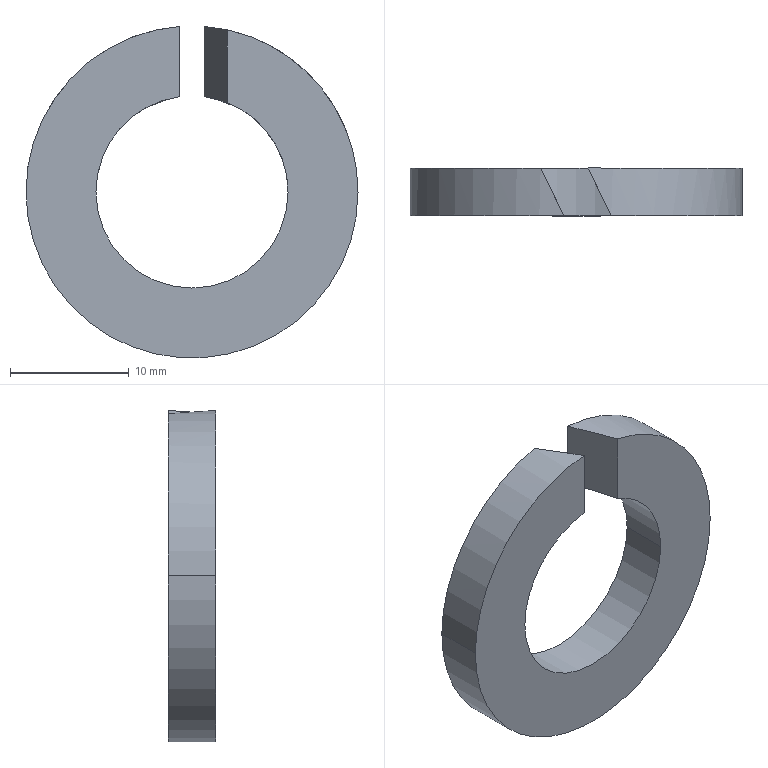Part | STEP file | ZZ24-M16 | 1 solid | 10 faces | box 28 x 4 x 27.962 mm | volume 1543 mm3 | cylinder 6 | plane 4 | commonest cylinder face diameters 16.2 x3 28 x3
STEP:
#1=CARTESIAN_POINT('',(0.,0.,0.));
#2=DIRECTION('',(0.,0.,1.));
#3=DIRECTION('',(1.,0.,0.));
#4=AXIS2_PLACEMENT_3D('',#1,#2,#3);
#5=CARTESIAN_POINT('',(2.975,0.,7.534));
#6=VERTEX_POINT('',#5);
#7=CARTESIAN_POINT('',(1.025,4.,8.035));
#8=VERTEX_POINT('',#7);
#9=CARTESIAN_POINT('',(2.975,0.,7.534));
#10=CARTESIAN_POINT('',(2.348,1.287,7.782));
#11=CARTESIAN_POINT('',(1.694,2.627,7.95));
#12=CARTESIAN_POINT('',(1.025,4.,8.035));
#13=(BOUNDED_CURVE()B_SPLINE_CURVE(3,(#9,#10,#11,#12),.UNSPECIFIED.,.F.,.F.)B_SPLINE_CURVE_WITH_KNOTS((4,4),(1.195,1.444),.PIECEWISE_BEZIER_KNOTS.)CURVE()GEOMETRIC_REPRESENTATION_ITEM()RATIONAL_B_SPLINE_CURVE((1.,0.9948,0.9948,1.))REPRESENTATION_ITEM(''));
#14=CARTESIAN_POINT('',(0.,4.,0.));
#15=DIRECTION('',(0.,-1.,0.));
#16=DIRECTION('',(-1.,0.,0.001512));
#17=AXIS2_PLACEMENT_3D('',#14,#15,#16);
#18=CYLINDRICAL_SURFACE('',#17,8.1);
#19=CARTESIAN_POINT('',(4.338,4.));
#20=CARTESIAN_POINT('',(4.342,3.942));
#21=CARTESIAN_POINT('',(4.349,3.825));
#22=CARTESIAN_POINT('',(4.36,3.649));
#23=CARTESIAN_POINT('',(4.372,3.472));
#24=CARTESIAN_POINT('',(4.383,3.295));
#25=CARTESIAN_POINT('',(4.394,3.117));
#26=CARTESIAN_POINT('',(4.406,2.937));
#27=CARTESIAN_POINT('',(4.417,2.758));
#28=CARTESIAN_POINT('',(4.428,2.577));
#29=CARTESIAN_POINT('',(4.44,2.396));
#30=CARTESIAN_POINT('',(4.451,2.214));
#31=CARTESIAN_POINT('',(4.462,2.032));
#32=CARTESIAN_POINT('',(4.474,1.849));
#33=CARTESIAN_POINT('',(4.485,1.666));
#34=CARTESIAN_POINT('',(4.496,1.482));
#35=CARTESIAN_POINT('',(4.508,1.298));
#36=CARTESIAN_POINT('',(4.519,1.114));
#37=CARTESIAN_POINT('',(4.53,0.9287));
#38=CARTESIAN_POINT('',(4.542,0.7434));
#39=CARTESIAN_POINT('',(4.553,0.5579));
#40=CARTESIAN_POINT('',(4.564,0.3721));
#41=CARTESIAN_POINT('',(4.576,0.1862));
#42=CARTESIAN_POINT('',(4.583,0.06207));
#43=CARTESIAN_POINT('',(4.587,0.));
#44=B_SPLINE_CURVE_WITH_KNOTS('',3,(#19,#20,#21,#22,#23,#24,#25,#26,#27,#28,#29,#30,#31,#32,#33,#34,#35,#36,#37,#38,#39,#40,#41,#42,#43),.UNSPECIFIED.,.F.,.F.,(4,1,1,1,1,1,1,1,1,1,1,1,1,1,1,1,1,1,1,1,1,1,4),(1.195,1.206,1.217,1.229,1.24,1.251,1.263,1.274,1.285,1.297,1.308,1.319,1.331,1.342,1.353,1.365,1.376,1.387,1.399,1.41,1.421,1.433,1.444),.QUASI_UNIFORM_KNOTS.);
#45=(GEOMETRIC_REPRESENTATION_CONTEXT(2)PARAMETRIC_REPRESENTATION_CONTEXT()REPRESENTATION_CONTEXT('',''));
#46=DEFINITIONAL_REPRESENTATION('',(#44),#45);
#47=PCURVE('',#18,#46);
#48=CARTESIAN_POINT('',(2.975,0.,14.));
#49=DIRECTION('',(-0.8988,-0.4384,0.));
#50=DIRECTION('',(0.4384,-0.8988,0.));
#51=AXIS2_PLACEMENT_3D('',#48,#49,#50);
#52=PLANE('',#51);
#53=CARTESIAN_POINT('',(0.,-6.466));
#54=CARTESIAN_POINT('',(-1.432,-6.218));
#55=CARTESIAN_POINT('',(-2.923,-6.05));
#56=CARTESIAN_POINT('',(-4.45,-5.965));
#57=(BOUNDED_CURVE()B_SPLINE_CURVE(3,(#53,#54,#55,#56),.UNSPECIFIED.,.F.,.F.)B_SPLINE_CURVE_WITH_KNOTS((4,4),(1.195,1.444),.PIECEWISE_BEZIER_KNOTS.)CURVE()GEOMETRIC_REPRESENTATION_ITEM()RATIONAL_B_SPLINE_CURVE((1.,0.9948,0.9948,1.))REPRESENTATION_ITEM(''));
#58=(GEOMETRIC_REPRESENTATION_CONTEXT(2)PARAMETRIC_REPRESENTATION_CONTEXT()REPRESENTATION_CONTEXT('',''));
#59=DEFINITIONAL_REPRESENTATION('',(#57),#58);
#60=PCURVE('',#52,#59);
#61=SURFACE_CURVE('',#13,(#47,#60),.PCURVE_S1.);
#62=EDGE_CURVE('',#6,#8,#61,.T.);
#63=ORIENTED_EDGE('',*,*,#62,.F.);
#64=CARTESIAN_POINT('',(8.1,0.,-0.01225));
#65=VERTEX_POINT('',#64);
#66=CARTESIAN_POINT('',(0.,0.,0.));
#67=DIRECTION('',(0.,1.,0.));
#68=DIRECTION('',(1.,0.,-0.001512));
#69=AXIS2_PLACEMENT_3D('',#66,#67,#68);
#70=CIRCLE('',#69,8.1);
#71=CARTESIAN_POINT('',(9.425,4.));
#72=DIRECTION('',(-1.,0.));
#73=VECTOR('',#72,1.);
#74=LINE('',#71,#73);
#75=(GEOMETRIC_REPRESENTATION_CONTEXT(2)PARAMETRIC_REPRESENTATION_CONTEXT()REPRESENTATION_CONTEXT('',''));
#76=DEFINITIONAL_REPRESENTATION('',(#74),#75);
#77=PCURVE('',#18,#76);
#78=CARTESIAN_POINT('',(0.,0.,0.));
#79=DIRECTION('',(0.,-1.,0.));
#80=DIRECTION('',(-1.,0.,0.001512));
#81=AXIS2_PLACEMENT_3D('',#78,#79,#80);
#82=PLANE('',#81);
#83=CARTESIAN_POINT('',(-8.1,0.));
#84=CARTESIAN_POINT('',(-8.1,14.03));
#85=CARTESIAN_POINT('',(4.05,7.015));
#86=CARTESIAN_POINT('',(16.2,0.));
#87=CARTESIAN_POINT('',(4.05,-7.015));
#88=CARTESIAN_POINT('',(-8.1,-14.03));
#89=CARTESIAN_POINT('',(-8.1,0.));
#90=(BOUNDED_CURVE()B_SPLINE_CURVE(2,(#83,#84,#85,#86,#87,#88,#89),.UNSPECIFIED.,.T.,.F.)B_SPLINE_CURVE_WITH_KNOTS((1,2,2,2,2,1),(-2.094,0.,2.094,4.189,6.283,8.378),.UNSPECIFIED.)CURVE()GEOMETRIC_REPRESENTATION_ITEM()RATIONAL_B_SPLINE_CURVE((1.,0.5,1.,0.5,1.,0.5,1.))REPRESENTATION_ITEM(''));
#91=(GEOMETRIC_REPRESENTATION_CONTEXT(2)PARAMETRIC_REPRESENTATION_CONTEXT()REPRESENTATION_CONTEXT('',''));
#92=DEFINITIONAL_REPRESENTATION('',(#90),#91);
#93=PCURVE('',#82,#92);
#94=SURFACE_CURVE('',#70,(#77,#93),.PCURVE_S1.);
#95=EDGE_CURVE('',#6,#65,#94,.T.);
#96=ORIENTED_EDGE('',*,*,#95,.T.);
#97=CARTESIAN_POINT('',(8.1,4.,-0.01225));
#98=VERTEX_POINT('',#97);
#99=CARTESIAN_POINT('',(8.1,4.,-0.01225));
#100=DIRECTION('',(0.,-1.,0.));
#101=VECTOR('',#100,1.);
#102=LINE('',#99,#101);
#103=CARTESIAN_POINT('',(3.142,0.));
#104=DIRECTION('',(0.,1.));
#105=VECTOR('',#104,1.);
#106=LINE('',#103,#105);
#107=(GEOMETRIC_REPRESENTATION_CONTEXT(2)PARAMETRIC_REPRESENTATION_CONTEXT()REPRESENTATION_CONTEXT('',''));
#108=DEFINITIONAL_REPRESENTATION('',(#106),#107);
#109=PCURVE('',#18,#108);
#110=CARTESIAN_POINT('',(0.,4.,0.));
#111=DIRECTION('',(0.,-1.,0.));
#112=DIRECTION('',(-1.,0.,0.001512));
#113=AXIS2_PLACEMENT_3D('',#110,#111,#112);
#114=CYLINDRICAL_SURFACE('',#113,8.1);
#115=CARTESIAN_POINT('',(3.142,0.));
#116=DIRECTION('',(0.,1.));
#117=VECTOR('',#116,1.);
#118=LINE('',#115,#117);
#119=(GEOMETRIC_REPRESENTATION_CONTEXT(2)PARAMETRIC_REPRESENTATION_CONTEXT()REPRESENTATION_CONTEXT('',''));
#120=DEFINITIONAL_REPRESENTATION('',(#118),#119);
#121=PCURVE('',#114,#120);
#122=SURFACE_CURVE('',#102,(#109,#121),.PCURVE_S1.);
#123=EDGE_CURVE('',#98,#65,#122,.T.);
#124=ORIENTED_EDGE('',*,*,#123,.F.);
#125=CARTESIAN_POINT('',(0.,4.,0.));
#126=DIRECTION('',(0.,-1.,0.));
#127=DIRECTION('',(-1.,0.,0.001512));
#128=AXIS2_PLACEMENT_3D('',#125,#126,#127);
#129=CIRCLE('',#128,8.1);
#130=CARTESIAN_POINT('',(0.,0.));
#131=DIRECTION('',(1.,0.));
#132=VECTOR('',#131,1.);
#133=LINE('',#130,#132);
#134=(GEOMETRIC_REPRESENTATION_CONTEXT(2)PARAMETRIC_REPRESENTATION_CONTEXT()REPRESENTATION_CONTEXT('',''));
#135=DEFINITIONAL_REPRESENTATION('',(#133),#134);
#136=PCURVE('',#18,#135);
#137=CARTESIAN_POINT('',(0.,4.,0.));
#138=DIRECTION('',(0.,1.,0.));
#139=DIRECTION('',(1.,0.,-0.001512));
#140=AXIS2_PLACEMENT_3D('',#137,#138,#139);
#141=PLANE('',#140);
#142=CARTESIAN_POINT('',(-8.1,0.));
#143=CARTESIAN_POINT('',(-8.1,14.03));
#144=CARTESIAN_POINT('',(4.05,7.015));
#145=CARTESIAN_POINT('',(16.2,0.));
#146=CARTESIAN_POINT('',(4.05,-7.015));
#147=CARTESIAN_POINT('',(-8.1,-14.03));
#148=CARTESIAN_POINT('',(-8.1,0.));
#149=(BOUNDED_CURVE()B_SPLINE_CURVE(2,(#142,#143,#144,#145,#146,#147,#148),.UNSPECIFIED.,.T.,.F.)B_SPLINE_CURVE_WITH_KNOTS((1,2,2,2,2,1),(-2.094,0.,2.094,4.189,6.283,8.378),.UNSPECIFIED.)CURVE()GEOMETRIC_REPRESENTATION_ITEM()RATIONAL_B_SPLINE_CURVE((1.,0.5,1.,0.5,1.,0.5,1.))REPRESENTATION_ITEM(''));
#150=(GEOMETRIC_REPRESENTATION_CONTEXT(2)PARAMETRIC_REPRESENTATION_CONTEXT()REPRESENTATION_CONTEXT('',''));
#151=DEFINITIONAL_REPRESENTATION('',(#149),#150);
#152=PCURVE('',#141,#151);
#153=SURFACE_CURVE('',#129,(#136,#152),.PCURVE_S1.);
#154=EDGE_CURVE('',#98,#8,#153,.T.);
#155=ORIENTED_EDGE('',*,*,#154,.T.);
#156=EDGE_LOOP('',(#63,#96,#124,#155));
#157=FACE_BOUND('',#156,.F.);
#158=ADVANCED_FACE('',(#157),#18,.F.);
#159=CARTESIAN_POINT('',(-8.1,0.,0.01225));
#160=VERTEX_POINT('',#159);
#161=CARTESIAN_POINT('',(0.,0.,0.));
#162=DIRECTION('',(0.,1.,0.));
#163=DIRECTION('',(1.,0.,-0.001512));
#164=AXIS2_PLACEMENT_3D('',#161,#162,#163);
#165=CIRCLE('',#164,8.1);
#166=CARTESIAN_POINT('',(3.142,4.));
#167=DIRECTION('',(-1.,0.));
#168=VECTOR('',#167,1.);
#169=LINE('',#166,#168);
#170=(GEOMETRIC_REPRESENTATION_CONTEXT(2)PARAMETRIC_REPRESENTATION_CONTEXT()REPRESENTATION_CONTEXT('',''));
#171=DEFINITIONAL_REPRESENTATION('',(#169),#170);
#172=PCURVE('',#114,#171);
#173=CARTESIAN_POINT('',(-8.1,0.));
#174=CARTESIAN_POINT('',(-8.1,14.03));
#175=CARTESIAN_POINT('',(4.05,7.015));
#176=CARTESIAN_POINT('',(16.2,0.));
#177=CARTESIAN_POINT('',(4.05,-7.015));
#178=CARTESIAN_POINT('',(-8.1,-14.03));
#179=CARTESIAN_POINT('',(-8.1,0.));
#180=(BOUNDED_CURVE()B_SPLINE_CURVE(2,(#173,#174,#175,#176,#177,#178,#179),.UNSPECIFIED.,.T.,.F.)B_SPLINE_CURVE_WITH_KNOTS((1,2,2,2,2,1),(-2.094,0.,2.094,4.189,6.283,8.378),.UNSPECIFIED.)CURVE()GEOMETRIC_REPRESENTATION_ITEM()RATIONAL_B_SPLINE_CURVE((1.,0.5,1.,0.5,1.,0.5,1.))REPRESENTATION_ITEM(''));
#181=(GEOMETRIC_REPRESENTATION_CONTEXT(2)PARAMETRIC_REPRESENTATION_CONTEXT()REPRESENTATION_CONTEXT('',''));
#182=DEFINITIONAL_REPRESENTATION('',(#180),#181);
#183=PCURVE('',#82,#182);
#184=SURFACE_CURVE('',#165,(#172,#183),.PCURVE_S1.);
#185=EDGE_CURVE('',#65,#160,#184,.T.);
#186=ORIENTED_EDGE('',*,*,#185,.T.);
#187=CARTESIAN_POINT('',(-8.1,4.,0.01225));
#188=VERTEX_POINT('',#187);
#189=CARTESIAN_POINT('',(-8.1,4.,0.01225));
#190=DIRECTION('',(0.,-1.,0.));
#191=VECTOR('',#190,1.);
#192=LINE('',#189,#191);
#193=CARTESIAN_POINT('',(0.,0.));
#194=DIRECTION('',(0.,1.));
#195=VECTOR('',#194,1.);
#196=LINE('',#193,#195);
#197=(GEOMETRIC_REPRESENTATION_CONTEXT(2)PARAMETRIC_REPRESENTATION_CONTEXT()REPRESENTATION_CONTEXT('',''));
#198=DEFINITIONAL_REPRESENTATION('',(#196),#197);
#199=PCURVE('',#114,#198);
#200=CARTESIAN_POINT('',(0.,4.,0.));
#201=DIRECTION('',(0.,-1.,0.));
#202=DIRECTION('',(-1.,0.,0.001512));
#203=AXIS2_PLACEMENT_3D('',#200,#201,#202);
#204=CYLINDRICAL_SURFACE('',#203,8.1);
#205=CARTESIAN_POINT('',(6.283,0.));
#206=DIRECTION('',(0.,1.));
#207=VECTOR('',#206,1.);
#208=LINE('',#205,#207);
#209=(GEOMETRIC_REPRESENTATION_CONTEXT(2)PARAMETRIC_REPRESENTATION_CONTEXT()REPRESENTATION_CONTEXT('',''));
#210=DEFINITIONAL_REPRESENTATION('',(#208),#209);
#211=PCURVE('',#204,#210);
#212=SURFACE_CURVE('',#192,(#199,#211),.PCURVE_S1.);
#213=EDGE_CURVE('',#188,#160,#212,.T.);
#214=ORIENTED_EDGE('',*,*,#213,.F.);
#215=CARTESIAN_POINT('',(0.,4.,0.));
#216=DIRECTION('',(0.,-1.,0.));
#217=DIRECTION('',(-1.,0.,0.001512));
#218=AXIS2_PLACEMENT_3D('',#215,#216,#217);
#219=CIRCLE('',#218,8.1);
#220=CARTESIAN_POINT('',(0.,0.));
#221=DIRECTION('',(1.,0.));
#222=VECTOR('',#221,1.);
#223=LINE('',#220,#222);
#224=(GEOMETRIC_REPRESENTATION_CONTEXT(2)PARAMETRIC_REPRESENTATION_CONTEXT()REPRESENTATION_CONTEXT('',''));
#225=DEFINITIONAL_REPRESENTATION('',(#223),#224);
#226=PCURVE('',#114,#225);
#227=CARTESIAN_POINT('',(-8.1,0.));
#228=CARTESIAN_POINT('',(-8.1,14.03));
#229=CARTESIAN_POINT('',(4.05,7.015));
#230=CARTESIAN_POINT('',(16.2,0.));
#231=CARTESIAN_POINT('',(4.05,-7.015));
#232=CARTESIAN_POINT('',(-8.1,-14.03));
#233=CARTESIAN_POINT('',(-8.1,0.));
#234=(BOUNDED_CURVE()B_SPLINE_CURVE(2,(#227,#228,#229,#230,#231,#232,#233),.UNSPECIFIED.,.T.,.F.)B_SPLINE_CURVE_WITH_KNOTS((1,2,2,2,2,1),(-2.094,0.,2.094,4.189,6.283,8.378),.UNSPECIFIED.)CURVE()GEOMETRIC_REPRESENTATION_ITEM()RATIONAL_B_SPLINE_CURVE((1.,0.5,1.,0.5,1.,0.5,1.))REPRESENTATION_ITEM(''));
#235=(GEOMETRIC_REPRESENTATION_CONTEXT(2)PARAMETRIC_REPRESENTATION_CONTEXT()REPRESENTATION_CONTEXT('',''));
#236=DEFINITIONAL_REPRESENTATION('',(#234),#235);
#237=PCURVE('',#141,#236);
#238=SURFACE_CURVE('',#219,(#226,#237),.PCURVE_S1.);
#239=EDGE_CURVE('',#188,#98,#238,.T.);
#240=ORIENTED_EDGE('',*,*,#239,.T.);
#241=ORIENTED_EDGE('',*,*,#123,.T.);
#242=EDGE_LOOP('',(#186,#214,#240,#241));
#243=FACE_BOUND('',#242,.F.);
#244=ADVANCED_FACE('',(#243),#114,.F.);
#245=CARTESIAN_POINT('',(-14.,4.,0.02117));
#246=VERTEX_POINT('',#245);
#247=CARTESIAN_POINT('',(14.,4.,-0.02117));
#248=VERTEX_POINT('',#247);
#249=CARTESIAN_POINT('',(0.,4.,0.));
#250=DIRECTION('',(0.,-1.,0.));
#251=DIRECTION('',(-1.,0.,0.001512));
#252=AXIS2_PLACEMENT_3D('',#249,#250,#251);
#253=CIRCLE('',#252,14.);
#254=CARTESIAN_POINT('',(0.,4.,0.));
#255=DIRECTION('',(0.,-1.,0.));
#256=DIRECTION('',(-1.,0.,0.001512));
#257=AXIS2_PLACEMENT_3D('',#254,#255,#256);
#258=CYLINDRICAL_SURFACE('',#257,14.);
#259=CARTESIAN_POINT('',(0.,0.));
#260=DIRECTION('',(1.,0.));
#261=VECTOR('',#260,1.);
#262=LINE('',#259,#261);
#263=(GEOMETRIC_REPRESENTATION_CONTEXT(2)PARAMETRIC_REPRESENTATION_CONTEXT()REPRESENTATION_CONTEXT('',''));
#264=DEFINITIONAL_REPRESENTATION('',(#262),#263);
#265=PCURVE('',#258,#264);
#266=CARTESIAN_POINT('',(-14.,0.));
#267=CARTESIAN_POINT('',(-14.,24.249));
#268=CARTESIAN_POINT('',(7.,12.124));
#269=CARTESIAN_POINT('',(28.,0.));
#270=CARTESIAN_POINT('',(7.,-12.124));
#271=CARTESIAN_POINT('',(-14.,-24.249));
#272=CARTESIAN_POINT('',(-14.,0.));
#273=(BOUNDED_CURVE()B_SPLINE_CURVE(2,(#266,#267,#268,#269,#270,#271,#272),.UNSPECIFIED.,.T.,.F.)B_SPLINE_CURVE_WITH_KNOTS((1,2,2,2,2,1),(-2.094,0.,2.094,4.189,6.283,8.378),.UNSPECIFIED.)CURVE()GEOMETRIC_REPRESENTATION_ITEM()RATIONAL_B_SPLINE_CURVE((1.,0.5,1.,0.5,1.,0.5,1.))REPRESENTATION_ITEM(''));
#274=(GEOMETRIC_REPRESENTATION_CONTEXT(2)PARAMETRIC_REPRESENTATION_CONTEXT()REPRESENTATION_CONTEXT('',''));
#275=DEFINITIONAL_REPRESENTATION('',(#273),#274);
#276=PCURVE('',#141,#275);
#277=SURFACE_CURVE('',#253,(#265,#276),.PCURVE_S1.);
#278=EDGE_CURVE('',#246,#248,#277,.T.);
#279=ORIENTED_EDGE('',*,*,#278,.T.);
#280=CARTESIAN_POINT('',(14.,0.,-0.02117));
#281=VERTEX_POINT('',#280);
#282=CARTESIAN_POINT('',(14.,4.,-0.02117));
#283=DIRECTION('',(0.,-1.,0.));
#284=VECTOR('',#283,1.);
#285=LINE('',#282,#284);
#286=CARTESIAN_POINT('',(3.142,0.));
#287=DIRECTION('',(0.,1.));
#288=VECTOR('',#287,1.);
#289=LINE('',#286,#288);
#290=(GEOMETRIC_REPRESENTATION_CONTEXT(2)PARAMETRIC_REPRESENTATION_CONTEXT()REPRESENTATION_CONTEXT('',''));
#291=DEFINITIONAL_REPRESENTATION('',(#289),#290);
#292=PCURVE('',#258,#291);
#293=CARTESIAN_POINT('',(0.,4.,0.));
#294=DIRECTION('',(0.,-1.,0.));
#295=DIRECTION('',(-1.,0.,0.001512));
#296=AXIS2_PLACEMENT_3D('',#293,#294,#295);
#297=CYLINDRICAL_SURFACE('',#296,14.);
#298=CARTESIAN_POINT('',(3.142,0.));
#299=DIRECTION('',(0.,1.));
#300=VECTOR('',#299,1.);
#301=LINE('',#298,#300);
#302=(GEOMETRIC_REPRESENTATION_CONTEXT(2)PARAMETRIC_REPRESENTATION_CONTEXT()REPRESENTATION_CONTEXT('',''));
#303=DEFINITIONAL_REPRESENTATION('',(#301),#302);
#304=PCURVE('',#297,#303);
#305=SURFACE_CURVE('',#285,(#292,#304),.PCURVE_S1.);
#306=EDGE_CURVE('',#248,#281,#305,.T.);
#307=ORIENTED_EDGE('',*,*,#306,.T.);
#308=CARTESIAN_POINT('',(-14.,0.,0.02117));
#309=VERTEX_POINT('',#308);
#310=CARTESIAN_POINT('',(0.,0.,0.));
#311=DIRECTION('',(0.,1.,0.));
#312=DIRECTION('',(1.,0.,-0.001512));
#313=AXIS2_PLACEMENT_3D('',#310,#311,#312);
#314=CIRCLE('',#313,14.);
#315=CARTESIAN_POINT('',(3.142,4.));
#316=DIRECTION('',(-1.,0.));
#317=VECTOR('',#316,1.);
#318=LINE('',#315,#317);
#319=(GEOMETRIC_REPRESENTATION_CONTEXT(2)PARAMETRIC_REPRESENTATION_CONTEXT()REPRESENTATION_CONTEXT('',''));
#320=DEFINITIONAL_REPRESENTATION('',(#318),#319);
#321=PCURVE('',#258,#320);
#322=CARTESIAN_POINT('',(-14.,0.));
#323=CARTESIAN_POINT('',(-14.,24.249));
#324=CARTESIAN_POINT('',(7.,12.124));
#325=CARTESIAN_POINT('',(28.,0.));
#326=CARTESIAN_POINT('',(7.,-12.124));
#327=CARTESIAN_POINT('',(-14.,-24.249));
#328=CARTESIAN_POINT('',(-14.,0.));
#329=(BOUNDED_CURVE()B_SPLINE_CURVE(2,(#322,#323,#324,#325,#326,#327,#328),.UNSPECIFIED.,.T.,.F.)B_SPLINE_CURVE_WITH_KNOTS((1,2,2,2,2,1),(-2.094,0.,2.094,4.189,6.283,8.378),.UNSPECIFIED.)CURVE()GEOMETRIC_REPRESENTATION_ITEM()RATIONAL_B_SPLINE_CURVE((1.,0.5,1.,0.5,1.,0.5,1.))REPRESENTATION_ITEM(''));
#330=(GEOMETRIC_REPRESENTATION_CONTEXT(2)PARAMETRIC_REPRESENTATION_CONTEXT()REPRESENTATION_CONTEXT('',''));
#331=DEFINITIONAL_REPRESENTATION('',(#329),#330);
#332=PCURVE('',#82,#331);
#333=SURFACE_CURVE('',#314,(#321,#332),.PCURVE_S1.);
#334=EDGE_CURVE('',#281,#309,#333,.T.);
#335=ORIENTED_EDGE('',*,*,#334,.T.);
#336=CARTESIAN_POINT('',(-14.,4.,0.02117));
#337=DIRECTION('',(0.,-1.,0.));
#338=VECTOR('',#337,1.);
#339=LINE('',#336,#338);
#340=CARTESIAN_POINT('',(0.,0.));
#341=DIRECTION('',(0.,1.));
#342=VECTOR('',#341,1.);
#343=LINE('',#340,#342);
#344=(GEOMETRIC_REPRESENTATION_CONTEXT(2)PARAMETRIC_REPRESENTATION_CONTEXT()REPRESENTATION_CONTEXT('',''));
#345=DEFINITIONAL_REPRESENTATION('',(#343),#344);
#346=PCURVE('',#258,#345);
#347=CARTESIAN_POINT('',(0.,4.,0.));
#348=DIRECTION('',(0.,-1.,0.));
#349=DIRECTION('',(-1.,0.,0.001512));
#350=AXIS2_PLACEMENT_3D('',#347,#348,#349);
#351=CYLINDRICAL_SURFACE('',#350,14.);
#352=CARTESIAN_POINT('',(6.283,0.));
#353=DIRECTION('',(0.,1.));
#354=VECTOR('',#353,1.);
#355=LINE('',#352,#354);
#356=(GEOMETRIC_REPRESENTATION_CONTEXT(2)PARAMETRIC_REPRESENTATION_CONTEXT()REPRESENTATION_CONTEXT('',''));
#357=DEFINITIONAL_REPRESENTATION('',(#355),#356);
#358=PCURVE('',#351,#357);
#359=SURFACE_CURVE('',#339,(#346,#358),.PCURVE_S1.);
#360=EDGE_CURVE('',#246,#309,#359,.T.);
#361=ORIENTED_EDGE('',*,*,#360,.F.);
#362=EDGE_LOOP('',(#279,#307,#335,#361));
#363=FACE_BOUND('',#362,.T.);
#364=ADVANCED_FACE('',(#363),#258,.T.);
#365=CARTESIAN_POINT('',(-2.975,4.,13.68));
#366=VERTEX_POINT('',#365);
#367=CARTESIAN_POINT('',(0.,4.,0.));
#368=DIRECTION('',(0.,-1.,0.));
#369=DIRECTION('',(-1.,0.,0.001512));
#370=AXIS2_PLACEMENT_3D('',#367,#368,#369);
#371=CIRCLE('',#370,14.);
#372=CARTESIAN_POINT('',(0.,0.));
#373=DIRECTION('',(1.,0.));
#374=VECTOR('',#373,1.);
#375=LINE('',#372,#374);
#376=(GEOMETRIC_REPRESENTATION_CONTEXT(2)PARAMETRIC_REPRESENTATION_CONTEXT()REPRESENTATION_CONTEXT('',''));
#377=DEFINITIONAL_REPRESENTATION('',(#375),#376);
#378=PCURVE('',#351,#377);
#379=CARTESIAN_POINT('',(-14.,0.));
#380=CARTESIAN_POINT('',(-14.,24.249));
#381=CARTESIAN_POINT('',(7.,12.124));
#382=CARTESIAN_POINT('',(28.,0.));
#383=CARTESIAN_POINT('',(7.,-12.124));
#384=CARTESIAN_POINT('',(-14.,-24.249));
#385=CARTESIAN_POINT('',(-14.,0.));
#386=(BOUNDED_CURVE()B_SPLINE_CURVE(2,(#379,#380,#381,#382,#383,#384,#385),.UNSPECIFIED.,.T.,.F.)B_SPLINE_CURVE_WITH_KNOTS((1,2,2,2,2,1),(-2.094,0.,2.094,4.189,6.283,8.378),.UNSPECIFIED.)CURVE()GEOMETRIC_REPRESENTATION_ITEM()RATIONAL_B_SPLINE_CURVE((1.,0.5,1.,0.5,1.,0.5,1.))REPRESENTATION_ITEM(''));
#387=(GEOMETRIC_REPRESENTATION_CONTEXT(2)PARAMETRIC_REPRESENTATION_CONTEXT()REPRESENTATION_CONTEXT('',''));
#388=DEFINITIONAL_REPRESENTATION('',(#386),#387);
#389=PCURVE('',#141,#388);
#390=SURFACE_CURVE('',#371,(#378,#389),.PCURVE_S1.);
#391=EDGE_CURVE('',#366,#246,#390,.T.);
#392=ORIENTED_EDGE('',*,*,#391,.T.);
#393=ORIENTED_EDGE('',*,*,#360,.T.);
#394=CARTESIAN_POINT('',(-1.025,0.,13.962));
#395=VERTEX_POINT('',#394);
#396=CARTESIAN_POINT('',(0.,0.,0.));
#397=DIRECTION('',(0.,1.,0.));
#398=DIRECTION('',(1.,0.,-0.001512));
#399=AXIS2_PLACEMENT_3D('',#396,#397,#398);
#400=CIRCLE('',#399,14.);
#401=CARTESIAN_POINT('',(9.425,4.));
#402=DIRECTION('',(-1.,0.));
#403=VECTOR('',#402,1.);
#404=LINE('',#401,#403);
#405=(GEOMETRIC_REPRESENTATION_CONTEXT(2)PARAMETRIC_REPRESENTATION_CONTEXT()REPRESENTATION_CONTEXT('',''));
#406=DEFINITIONAL_REPRESENTATION('',(#404),#405);
#407=PCURVE('',#351,#406);
#408=CARTESIAN_POINT('',(-14.,0.));
#409=CARTESIAN_POINT('',(-14.,24.249));
#410=CARTESIAN_POINT('',(7.,12.124));
#411=CARTESIAN_POINT('',(28.,0.));
#412=CARTESIAN_POINT('',(7.,-12.124));
#413=CARTESIAN_POINT('',(-14.,-24.249));
#414=CARTESIAN_POINT('',(-14.,0.));
#415=(BOUNDED_CURVE()B_SPLINE_CURVE(2,(#408,#409,#410,#411,#412,#413,#414),.UNSPECIFIED.,.T.,.F.)B_SPLINE_CURVE_WITH_KNOTS((1,2,2,2,2,1),(-2.094,0.,2.094,4.189,6.283,8.378),.UNSPECIFIED.)CURVE()GEOMETRIC_REPRESENTATION_ITEM()RATIONAL_B_SPLINE_CURVE((1.,0.5,1.,0.5,1.,0.5,1.))REPRESENTATION_ITEM(''));
#416=(GEOMETRIC_REPRESENTATION_CONTEXT(2)PARAMETRIC_REPRESENTATION_CONTEXT()REPRESENTATION_CONTEXT('',''));
#417=DEFINITIONAL_REPRESENTATION('',(#415),#416);
#418=PCURVE('',#82,#417);
#419=SURFACE_CURVE('',#400,(#407,#418),.PCURVE_S1.);
#420=EDGE_CURVE('',#309,#395,#419,.T.);
#421=ORIENTED_EDGE('',*,*,#420,.T.);
#422=CARTESIAN_POINT('',(-1.025,0.,13.962));
#423=CARTESIAN_POINT('',(-1.681,1.346,13.914));
#424=CARTESIAN_POINT('',(-2.332,2.681,13.82));
#425=CARTESIAN_POINT('',(-2.975,4.,13.68));
#426=(BOUNDED_CURVE()B_SPLINE_CURVE(3,(#422,#423,#424,#425),.UNSPECIFIED.,.F.,.F.)B_SPLINE_CURVE_WITH_KNOTS((4,4),(1.644,1.785),.PIECEWISE_BEZIER_KNOTS.)CURVE()GEOMETRIC_REPRESENTATION_ITEM()RATIONAL_B_SPLINE_CURVE((1.,0.9983,0.9983,1.))REPRESENTATION_ITEM(''));
#427=CARTESIAN_POINT('',(4.787,4.));
#428=CARTESIAN_POINT('',(4.789,3.939));
#429=CARTESIAN_POINT('',(4.794,3.817));
#430=CARTESIAN_POINT('',(4.8,3.634));
#431=CARTESIAN_POINT('',(4.806,3.451));
#432=CARTESIAN_POINT('',(4.813,3.268));
#433=CARTESIAN_POINT('',(4.819,3.085));
#434=CARTESIAN_POINT('',(4.826,2.902));
#435=CARTESIAN_POINT('',(4.832,2.719));
#436=CARTESIAN_POINT('',(4.838,2.537));
#437=CARTESIAN_POINT('',(4.845,2.354));
#438=CARTESIAN_POINT('',(4.851,2.172));
#439=CARTESIAN_POINT('',(4.858,1.99));
#440=CARTESIAN_POINT('',(4.864,1.808));
#441=CARTESIAN_POINT('',(4.87,1.626));
#442=CARTESIAN_POINT('',(4.877,1.444));
#443=CARTESIAN_POINT('',(4.883,1.263));
#444=CARTESIAN_POINT('',(4.89,1.082));
#445=CARTESIAN_POINT('',(4.896,0.9009));
#446=CARTESIAN_POINT('',(4.902,0.7202));
#447=CARTESIAN_POINT('',(4.909,0.5398));
#448=CARTESIAN_POINT('',(4.915,0.3596));
#449=CARTESIAN_POINT('',(4.922,0.1796));
#450=CARTESIAN_POINT('',(4.926,0.05984));
#451=CARTESIAN_POINT('',(4.928,0.));
#452=B_SPLINE_CURVE_WITH_KNOTS('',3,(#427,#428,#429,#430,#431,#432,#433,#434,#435,#436,#437,#438,#439,#440,#441,#442,#443,#444,#445,#446,#447,#448,#449,#450,#451),.UNSPECIFIED.,.F.,.F.,(4,1,1,1,1,1,1,1,1,1,1,1,1,1,1,1,1,1,1,1,1,1,4),(1.644,1.65,1.657,1.663,1.67,1.676,1.682,1.689,1.695,1.702,1.708,1.715,1.721,1.727,1.734,1.74,1.747,1.753,1.759,1.766,1.772,1.779,1.785),.QUASI_UNIFORM_KNOTS.);
#453=(GEOMETRIC_REPRESENTATION_CONTEXT(2)PARAMETRIC_REPRESENTATION_CONTEXT()REPRESENTATION_CONTEXT('',''));
#454=DEFINITIONAL_REPRESENTATION('',(#452),#453);
#455=PCURVE('',#351,#454);
#456=CARTESIAN_POINT('',(-2.975,4.,14.));
#457=DIRECTION('',(0.8988,0.4384,0.));
#458=DIRECTION('',(-0.4384,0.8988,0.));
#459=AXIS2_PLACEMENT_3D('',#456,#457,#458);
#460=PLANE('',#459);
#461=CARTESIAN_POINT('',(-4.45,-0.03754));
#462=CARTESIAN_POINT('',(-2.953,-0.0857));
#463=CARTESIAN_POINT('',(-1.467,-0.18));
#464=CARTESIAN_POINT('',(0.,-0.3198));
#465=(BOUNDED_CURVE()B_SPLINE_CURVE(3,(#461,#462,#463,#464),.UNSPECIFIED.,.F.,.F.)B_SPLINE_CURVE_WITH_KNOTS((4,4),(1.644,1.785),.PIECEWISE_BEZIER_KNOTS.)CURVE()GEOMETRIC_REPRESENTATION_ITEM()RATIONAL_B_SPLINE_CURVE((1.,0.9983,0.9983,1.))REPRESENTATION_ITEM(''));
#466=(GEOMETRIC_REPRESENTATION_CONTEXT(2)PARAMETRIC_REPRESENTATION_CONTEXT()REPRESENTATION_CONTEXT('',''));
#467=DEFINITIONAL_REPRESENTATION('',(#465),#466);
#468=PCURVE('',#460,#467);
#469=SURFACE_CURVE('',#426,(#455,#468),.PCURVE_S1.);
#470=EDGE_CURVE('',#395,#366,#469,.T.);
#471=ORIENTED_EDGE('',*,*,#470,.T.);
#472=EDGE_LOOP('',(#392,#393,#421,#471));
#473=FACE_BOUND('',#472,.T.);
#474=ADVANCED_FACE('',(#473),#351,.T.);
#475=CARTESIAN_POINT('',(-1.025,0.,8.035));
#476=VERTEX_POINT('',#475);
#477=CARTESIAN_POINT('',(-1.025,0.,14.));
#478=DIRECTION('',(0.,0.,-1.));
#479=VECTOR('',#478,1.);
#480=LINE('',#477,#479);
#481=CARTESIAN_POINT('',(1.046,-13.998));
#482=DIRECTION('',(-0.001512,1.));
#483=VECTOR('',#482,1.);
#484=LINE('',#481,#483);
#485=(GEOMETRIC_REPRESENTATION_CONTEXT(2)PARAMETRIC_REPRESENTATION_CONTEXT()REPRESENTATION_CONTEXT('',''));
#486=DEFINITIONAL_REPRESENTATION('',(#484),#485);
#487=PCURVE('',#82,#486);
#488=CARTESIAN_POINT('',(-4.45,0.));
#489=DIRECTION('',(0.,-1.));
#490=VECTOR('',#489,1.);
#491=LINE('',#488,#490);
#492=(GEOMETRIC_REPRESENTATION_CONTEXT(2)PARAMETRIC_REPRESENTATION_CONTEXT()REPRESENTATION_CONTEXT('',''));
#493=DEFINITIONAL_REPRESENTATION('',(#491),#492);
#494=PCURVE('',#460,#493);
#495=SURFACE_CURVE('',#480,(#487,#494),.PCURVE_S1.);
#496=EDGE_CURVE('',#395,#476,#495,.T.);
#497=ORIENTED_EDGE('',*,*,#496,.F.);
#498=ORIENTED_EDGE('',*,*,#420,.F.);
#499=ORIENTED_EDGE('',*,*,#334,.F.);
#500=CARTESIAN_POINT('',(2.975,0.,13.68));
#501=VERTEX_POINT('',#500);
#502=CARTESIAN_POINT('',(0.,0.,0.));
#503=DIRECTION('',(0.,1.,0.));
#504=DIRECTION('',(1.,0.,-0.001512));
#505=AXIS2_PLACEMENT_3D('',#502,#503,#504);
#506=CIRCLE('',#505,14.);
#507=CARTESIAN_POINT('',(-14.,0.));
#508=CARTESIAN_POINT('',(-14.,24.249));
#509=CARTESIAN_POINT('',(7.,12.124));
#510=CARTESIAN_POINT('',(28.,0.));
#511=CARTESIAN_POINT('',(7.,-12.124));
#512=CARTESIAN_POINT('',(-14.,-24.249));
#513=CARTESIAN_POINT('',(-14.,0.));
#514=(BOUNDED_CURVE()B_SPLINE_CURVE(2,(#507,#508,#509,#510,#511,#512,#513),.UNSPECIFIED.,.T.,.F.)B_SPLINE_CURVE_WITH_KNOTS((1,2,2,2,2,1),(-2.094,0.,2.094,4.189,6.283,8.378),.UNSPECIFIED.)CURVE()GEOMETRIC_REPRESENTATION_ITEM()RATIONAL_B_SPLINE_CURVE((1.,0.5,1.,0.5,1.,0.5,1.))REPRESENTATION_ITEM(''));
#515=(GEOMETRIC_REPRESENTATION_CONTEXT(2)PARAMETRIC_REPRESENTATION_CONTEXT()REPRESENTATION_CONTEXT('',''));
#516=DEFINITIONAL_REPRESENTATION('',(#514),#515);
#517=PCURVE('',#82,#516);
#518=CARTESIAN_POINT('',(9.425,4.));
#519=DIRECTION('',(-1.,0.));
#520=VECTOR('',#519,1.);
#521=LINE('',#518,#520);
#522=(GEOMETRIC_REPRESENTATION_CONTEXT(2)PARAMETRIC_REPRESENTATION_CONTEXT()REPRESENTATION_CONTEXT('',''));
#523=DEFINITIONAL_REPRESENTATION('',(#521),#522);
#524=PCURVE('',#297,#523);
#525=SURFACE_CURVE('',#506,(#517,#524),.PCURVE_S1.);
#526=EDGE_CURVE('',#501,#281,#525,.T.);
#527=ORIENTED_EDGE('',*,*,#526,.F.);
#528=CARTESIAN_POINT('',(2.975,0.,14.));
#529=DIRECTION('',(0.,0.,-1.));
#530=VECTOR('',#529,1.);
#531=LINE('',#528,#530);
#532=CARTESIAN_POINT('',(-2.954,-14.004));
#533=DIRECTION('',(-0.001512,1.));
#534=VECTOR('',#533,1.);
#535=LINE('',#532,#534);
#536=(GEOMETRIC_REPRESENTATION_CONTEXT(2)PARAMETRIC_REPRESENTATION_CONTEXT()REPRESENTATION_CONTEXT('',''));
#537=DEFINITIONAL_REPRESENTATION('',(#535),#536);
#538=PCURVE('',#82,#537);
#539=CARTESIAN_POINT('',(0.,0.));
#540=DIRECTION('',(0.,-1.));
#541=VECTOR('',#540,1.);
#542=LINE('',#539,#541);
#543=(GEOMETRIC_REPRESENTATION_CONTEXT(2)PARAMETRIC_REPRESENTATION_CONTEXT()REPRESENTATION_CONTEXT('',''));
#544=DEFINITIONAL_REPRESENTATION('',(#542),#543);
#545=PCURVE('',#52,#544);
#546=SURFACE_CURVE('',#531,(#538,#545),.PCURVE_S1.);
#547=EDGE_CURVE('',#501,#6,#546,.T.);
#548=ORIENTED_EDGE('',*,*,#547,.T.);
#549=ORIENTED_EDGE('',*,*,#95,.T.);
#550=ORIENTED_EDGE('',*,*,#185,.T.);
#551=CARTESIAN_POINT('',(0.,0.,0.));
#552=DIRECTION('',(0.,1.,0.));
#553=DIRECTION('',(1.,0.,-0.001512));
#554=AXIS2_PLACEMENT_3D('',#551,#552,#553);
#555=CIRCLE('',#554,8.1);
#556=CARTESIAN_POINT('',(-8.1,0.));
#557=CARTESIAN_POINT('',(-8.1,14.03));
#558=CARTESIAN_POINT('',(4.05,7.015));
#559=CARTESIAN_POINT('',(16.2,0.));
#560=CARTESIAN_POINT('',(4.05,-7.015));
#561=CARTESIAN_POINT('',(-8.1,-14.03));
#562=CARTESIAN_POINT('',(-8.1,0.));
#563=(BOUNDED_CURVE()B_SPLINE_CURVE(2,(#556,#557,#558,#559,#560,#561,#562),.UNSPECIFIED.,.T.,.F.)B_SPLINE_CURVE_WITH_KNOTS((1,2,2,2,2,1),(-2.094,0.,2.094,4.189,6.283,8.378),.UNSPECIFIED.)CURVE()GEOMETRIC_REPRESENTATION_ITEM()RATIONAL_B_SPLINE_CURVE((1.,0.5,1.,0.5,1.,0.5,1.))REPRESENTATION_ITEM(''));
#564=(GEOMETRIC_REPRESENTATION_CONTEXT(2)PARAMETRIC_REPRESENTATION_CONTEXT()REPRESENTATION_CONTEXT('',''));
#565=DEFINITIONAL_REPRESENTATION('',(#563),#564);
#566=PCURVE('',#82,#565);
#567=CARTESIAN_POINT('',(9.425,4.));
#568=DIRECTION('',(-1.,0.));
#569=VECTOR('',#568,1.);
#570=LINE('',#567,#569);
#571=(GEOMETRIC_REPRESENTATION_CONTEXT(2)PARAMETRIC_REPRESENTATION_CONTEXT()REPRESENTATION_CONTEXT('',''));
#572=DEFINITIONAL_REPRESENTATION('',(#570),#571);
#573=PCURVE('',#204,#572);
#574=SURFACE_CURVE('',#555,(#566,#573),.PCURVE_S1.);
#575=EDGE_CURVE('',#160,#476,#574,.T.);
#576=ORIENTED_EDGE('',*,*,#575,.T.);
#577=EDGE_LOOP('',(#497,#498,#499,#527,#548,#549,#550,#576));
#578=FACE_BOUND('',#577,.T.);
#579=ADVANCED_FACE('',(#578),#82,.T.);
#580=CARTESIAN_POINT('',(1.025,4.,13.962));
#581=VERTEX_POINT('',#580);
#582=CARTESIAN_POINT('',(1.025,4.,14.));
#583=DIRECTION('',(0.,0.,-1.));
#584=VECTOR('',#583,1.);
#585=LINE('',#582,#584);
#586=CARTESIAN_POINT('',(1.003,-14.002));
#587=DIRECTION('',(0.001512,1.));
#588=VECTOR('',#587,1.);
#589=LINE('',#586,#588);
#590=(GEOMETRIC_REPRESENTATION_CONTEXT(2)PARAMETRIC_REPRESENTATION_CONTEXT()REPRESENTATION_CONTEXT('',''));
#591=DEFINITIONAL_REPRESENTATION('',(#589),#590);
#592=PCURVE('',#141,#591);
#593=CARTESIAN_POINT('',(-4.45,0.));
#594=DIRECTION('',(0.,-1.));
#595=VECTOR('',#594,1.);
#596=LINE('',#593,#595);
#597=(GEOMETRIC_REPRESENTATION_CONTEXT(2)PARAMETRIC_REPRESENTATION_CONTEXT()REPRESENTATION_CONTEXT('',''));
#598=DEFINITIONAL_REPRESENTATION('',(#596),#597);
#599=PCURVE('',#52,#598);
#600=SURFACE_CURVE('',#585,(#592,#599),.PCURVE_S1.);
#601=EDGE_CURVE('',#581,#8,#600,.T.);
#602=ORIENTED_EDGE('',*,*,#601,.F.);
#603=CARTESIAN_POINT('',(0.,4.,0.));
#604=DIRECTION('',(0.,-1.,0.));
#605=DIRECTION('',(-1.,0.,0.001512));
#606=AXIS2_PLACEMENT_3D('',#603,#604,#605);
#607=CIRCLE('',#606,14.);
#608=CARTESIAN_POINT('',(-14.,0.));
#609=CARTESIAN_POINT('',(-14.,24.249));
#610=CARTESIAN_POINT('',(7.,12.124));
#611=CARTESIAN_POINT('',(28.,0.));
#612=CARTESIAN_POINT('',(7.,-12.124));
#613=CARTESIAN_POINT('',(-14.,-24.249));
#614=CARTESIAN_POINT('',(-14.,0.));
#615=(BOUNDED_CURVE()B_SPLINE_CURVE(2,(#608,#609,#610,#611,#612,#613,#614),.UNSPECIFIED.,.T.,.F.)B_SPLINE_CURVE_WITH_KNOTS((1,2,2,2,2,1),(-2.094,0.,2.094,4.189,6.283,8.378),.UNSPECIFIED.)CURVE()GEOMETRIC_REPRESENTATION_ITEM()RATIONAL_B_SPLINE_CURVE((1.,0.5,1.,0.5,1.,0.5,1.))REPRESENTATION_ITEM(''));
#616=(GEOMETRIC_REPRESENTATION_CONTEXT(2)PARAMETRIC_REPRESENTATION_CONTEXT()REPRESENTATION_CONTEXT('',''));
#617=DEFINITIONAL_REPRESENTATION('',(#615),#616);
#618=PCURVE('',#141,#617);
#619=CARTESIAN_POINT('',(0.,0.));
#620=DIRECTION('',(1.,0.));
#621=VECTOR('',#620,1.);
#622=LINE('',#619,#621);
#623=(GEOMETRIC_REPRESENTATION_CONTEXT(2)PARAMETRIC_REPRESENTATION_CONTEXT()REPRESENTATION_CONTEXT('',''));
#624=DEFINITIONAL_REPRESENTATION('',(#622),#623);
#625=PCURVE('',#297,#624);
#626=SURFACE_CURVE('',#607,(#618,#625),.PCURVE_S1.);
#627=EDGE_CURVE('',#248,#581,#626,.T.);
#628=ORIENTED_EDGE('',*,*,#627,.F.);
#629=ORIENTED_EDGE('',*,*,#278,.F.);
#630=ORIENTED_EDGE('',*,*,#391,.F.);
#631=CARTESIAN_POINT('',(-2.975,4.,7.534));
#632=VERTEX_POINT('',#631);
#633=CARTESIAN_POINT('',(-2.975,4.,14.));
#634=DIRECTION('',(0.,0.,-1.));
#635=VECTOR('',#634,1.);
#636=LINE('',#633,#635);
#637=CARTESIAN_POINT('',(-2.997,-13.995));
#638=DIRECTION('',(0.001512,1.));
#639=VECTOR('',#638,1.);
#640=LINE('',#637,#639);
#641=(GEOMETRIC_REPRESENTATION_CONTEXT(2)PARAMETRIC_REPRESENTATION_CONTEXT()REPRESENTATION_CONTEXT('',''));
#642=DEFINITIONAL_REPRESENTATION('',(#640),#641);
#643=PCURVE('',#141,#642);
#644=CARTESIAN_POINT('',(0.,0.));
#645=DIRECTION('',(0.,-1.));
#646=VECTOR('',#645,1.);
#647=LINE('',#644,#646);
#648=(GEOMETRIC_REPRESENTATION_CONTEXT(2)PARAMETRIC_REPRESENTATION_CONTEXT()REPRESENTATION_CONTEXT('',''));
#649=DEFINITIONAL_REPRESENTATION('',(#647),#648);
#650=PCURVE('',#460,#649);
#651=SURFACE_CURVE('',#636,(#643,#650),.PCURVE_S1.);
#652=EDGE_CURVE('',#366,#632,#651,.T.);
#653=ORIENTED_EDGE('',*,*,#652,.T.);
#654=CARTESIAN_POINT('',(0.,4.,0.));
#655=DIRECTION('',(0.,-1.,0.));
#656=DIRECTION('',(-1.,0.,0.001512));
#657=AXIS2_PLACEMENT_3D('',#654,#655,#656);
#658=CIRCLE('',#657,8.1);
#659=CARTESIAN_POINT('',(-8.1,0.));
#660=CARTESIAN_POINT('',(-8.1,14.03));
#661=CARTESIAN_POINT('',(4.05,7.015));
#662=CARTESIAN_POINT('',(16.2,0.));
#663=CARTESIAN_POINT('',(4.05,-7.015));
#664=CARTESIAN_POINT('',(-8.1,-14.03));
#665=CARTESIAN_POINT('',(-8.1,0.));
#666=(BOUNDED_CURVE()B_SPLINE_CURVE(2,(#659,#660,#661,#662,#663,#664,#665),.UNSPECIFIED.,.T.,.F.)B_SPLINE_CURVE_WITH_KNOTS((1,2,2,2,2,1),(-2.094,0.,2.094,4.189,6.283,8.378),.UNSPECIFIED.)CURVE()GEOMETRIC_REPRESENTATION_ITEM()RATIONAL_B_SPLINE_CURVE((1.,0.5,1.,0.5,1.,0.5,1.))REPRESENTATION_ITEM(''));
#667=(GEOMETRIC_REPRESENTATION_CONTEXT(2)PARAMETRIC_REPRESENTATION_CONTEXT()REPRESENTATION_CONTEXT('',''));
#668=DEFINITIONAL_REPRESENTATION('',(#666),#667);
#669=PCURVE('',#141,#668);
#670=CARTESIAN_POINT('',(0.,0.));
#671=DIRECTION('',(1.,0.));
#672=VECTOR('',#671,1.);
#673=LINE('',#670,#672);
#674=(GEOMETRIC_REPRESENTATION_CONTEXT(2)PARAMETRIC_REPRESENTATION_CONTEXT()REPRESENTATION_CONTEXT('',''));
#675=DEFINITIONAL_REPRESENTATION('',(#673),#674);
#676=PCURVE('',#204,#675);
#677=SURFACE_CURVE('',#658,(#669,#676),.PCURVE_S1.);
#678=EDGE_CURVE('',#632,#188,#677,.T.);
#679=ORIENTED_EDGE('',*,*,#678,.T.);
#680=ORIENTED_EDGE('',*,*,#239,.T.);
#681=ORIENTED_EDGE('',*,*,#154,.T.);
#682=EDGE_LOOP('',(#602,#628,#629,#630,#653,#679,#680,#681));
#683=FACE_BOUND('',#682,.T.);
#684=ADVANCED_FACE('',(#683),#141,.T.);
#685=ORIENTED_EDGE('',*,*,#306,.F.);
#686=ORIENTED_EDGE('',*,*,#627,.T.);
#687=CARTESIAN_POINT('',(1.025,4.,13.962));
#688=CARTESIAN_POINT('',(1.681,2.654,13.914));
#689=CARTESIAN_POINT('',(2.332,1.319,13.82));
#690=CARTESIAN_POINT('',(2.975,0.,13.68));
#691=(BOUNDED_CURVE()B_SPLINE_CURVE(3,(#687,#688,#689,#690),.UNSPECIFIED.,.F.,.F.)B_SPLINE_CURVE_WITH_KNOTS((4,4),(4.786,4.927),.PIECEWISE_BEZIER_KNOTS.)CURVE()GEOMETRIC_REPRESENTATION_ITEM()RATIONAL_B_SPLINE_CURVE((1.,0.9983,0.9983,1.))REPRESENTATION_ITEM(''));
#692=CARTESIAN_POINT('',(4.641,0.));
#693=CARTESIAN_POINT('',(4.639,0.06107));
#694=CARTESIAN_POINT('',(4.634,0.1832));
#695=CARTESIAN_POINT('',(4.628,0.3663));
#696=CARTESIAN_POINT('',(4.621,0.5494));
#697=CARTESIAN_POINT('',(4.615,0.7324));
#698=CARTESIAN_POINT('',(4.609,0.9153));
#699=CARTESIAN_POINT('',(4.602,1.098));
#700=CARTESIAN_POINT('',(4.596,1.281));
#701=CARTESIAN_POINT('',(4.589,1.463));
#702=CARTESIAN_POINT('',(4.583,1.646));
#703=CARTESIAN_POINT('',(4.577,1.828));
#704=CARTESIAN_POINT('',(4.57,2.01));
#705=CARTESIAN_POINT('',(4.564,2.192));
#706=CARTESIAN_POINT('',(4.557,2.374));
#707=CARTESIAN_POINT('',(4.551,2.556));
#708=CARTESIAN_POINT('',(4.545,2.737));
#709=CARTESIAN_POINT('',(4.538,2.918));
#710=CARTESIAN_POINT('',(4.532,3.099));
#711=CARTESIAN_POINT('',(4.525,3.28));
#712=CARTESIAN_POINT('',(4.519,3.46));
#713=CARTESIAN_POINT('',(4.513,3.64));
#714=CARTESIAN_POINT('',(4.506,3.82));
#715=CARTESIAN_POINT('',(4.502,3.94));
#716=CARTESIAN_POINT('',(4.5,4.));
#717=B_SPLINE_CURVE_WITH_KNOTS('',3,(#692,#693,#694,#695,#696,#697,#698,#699,#700,#701,#702,#703,#704,#705,#706,#707,#708,#709,#710,#711,#712,#713,#714,#715,#716),.UNSPECIFIED.,.F.,.F.,(4,1,1,1,1,1,1,1,1,1,1,1,1,1,1,1,1,1,1,1,1,1,4),(4.786,4.792,4.798,4.805,4.811,4.818,4.824,4.83,4.837,4.843,4.85,4.856,4.863,4.869,4.875,4.882,4.888,4.895,4.901,4.907,4.914,4.92,4.927),.QUASI_UNIFORM_KNOTS.);
#718=(GEOMETRIC_REPRESENTATION_CONTEXT(2)PARAMETRIC_REPRESENTATION_CONTEXT()REPRESENTATION_CONTEXT('',''));
#719=DEFINITIONAL_REPRESENTATION('',(#717),#718);
#720=PCURVE('',#297,#719);
#721=CARTESIAN_POINT('',(-4.45,-0.03754));
#722=CARTESIAN_POINT('',(-2.953,-0.0857));
#723=CARTESIAN_POINT('',(-1.467,-0.18));
#724=CARTESIAN_POINT('',(0.,-0.3198));
#725=(BOUNDED_CURVE()B_SPLINE_CURVE(3,(#721,#722,#723,#724),.UNSPECIFIED.,.F.,.F.)B_SPLINE_CURVE_WITH_KNOTS((4,4),(4.786,4.927),.PIECEWISE_BEZIER_KNOTS.)CURVE()GEOMETRIC_REPRESENTATION_ITEM()RATIONAL_B_SPLINE_CURVE((1.,0.9983,0.9983,1.))REPRESENTATION_ITEM(''));
#726=(GEOMETRIC_REPRESENTATION_CONTEXT(2)PARAMETRIC_REPRESENTATION_CONTEXT()REPRESENTATION_CONTEXT('',''));
#727=DEFINITIONAL_REPRESENTATION('',(#725),#726);
#728=PCURVE('',#52,#727);
#729=SURFACE_CURVE('',#691,(#720,#728),.PCURVE_S1.);
#730=EDGE_CURVE('',#581,#501,#729,.T.);
#731=ORIENTED_EDGE('',*,*,#730,.T.);
#732=ORIENTED_EDGE('',*,*,#526,.T.);
#733=EDGE_LOOP('',(#685,#686,#731,#732));
#734=FACE_BOUND('',#733,.T.);
#735=ADVANCED_FACE('',(#734),#297,.T.);
#736=ORIENTED_EDGE('',*,*,#601,.T.);
#737=ORIENTED_EDGE('',*,*,#62,.F.);
#738=ORIENTED_EDGE('',*,*,#547,.F.);
#739=ORIENTED_EDGE('',*,*,#730,.F.);
#740=EDGE_LOOP('',(#736,#737,#738,#739));
#741=FACE_BOUND('',#740,.T.);
#742=ADVANCED_FACE('',(#741),#52,.T.);
#743=ORIENTED_EDGE('',*,*,#496,.T.);
#744=CARTESIAN_POINT('',(-2.975,4.,7.534));
#745=CARTESIAN_POINT('',(-2.348,2.713,7.782));
#746=CARTESIAN_POINT('',(-1.694,1.373,7.95));
#747=CARTESIAN_POINT('',(-1.025,0.,8.035));
#748=(BOUNDED_CURVE()B_SPLINE_CURVE(3,(#744,#745,#746,#747),.UNSPECIFIED.,.F.,.F.)B_SPLINE_CURVE_WITH_KNOTS((4,4),(4.336,4.586),.PIECEWISE_BEZIER_KNOTS.)CURVE()GEOMETRIC_REPRESENTATION_ITEM()RATIONAL_B_SPLINE_CURVE((1.,0.9948,0.9948,1.))REPRESENTATION_ITEM(''));
#749=CARTESIAN_POINT('',(0.,-6.466));
#750=CARTESIAN_POINT('',(-1.432,-6.218));
#751=CARTESIAN_POINT('',(-2.923,-6.05));
#752=CARTESIAN_POINT('',(-4.45,-5.965));
#753=(BOUNDED_CURVE()B_SPLINE_CURVE(3,(#749,#750,#751,#752),.UNSPECIFIED.,.F.,.F.)B_SPLINE_CURVE_WITH_KNOTS((4,4),(4.336,4.586),.PIECEWISE_BEZIER_KNOTS.)CURVE()GEOMETRIC_REPRESENTATION_ITEM()RATIONAL_B_SPLINE_CURVE((1.,0.9948,0.9948,1.))REPRESENTATION_ITEM(''));
#754=(GEOMETRIC_REPRESENTATION_CONTEXT(2)PARAMETRIC_REPRESENTATION_CONTEXT()REPRESENTATION_CONTEXT('',''));
#755=DEFINITIONAL_REPRESENTATION('',(#753),#754);
#756=PCURVE('',#460,#755);
#757=CARTESIAN_POINT('',(5.09,0.));
#758=CARTESIAN_POINT('',(5.086,0.0582));
#759=CARTESIAN_POINT('',(5.079,0.1749));
#760=CARTESIAN_POINT('',(5.067,0.3508));
#761=CARTESIAN_POINT('',(5.056,0.5276));
#762=CARTESIAN_POINT('',(5.045,0.7051));
#763=CARTESIAN_POINT('',(5.033,0.8835));
#764=CARTESIAN_POINT('',(5.022,1.063));
#765=CARTESIAN_POINT('',(5.011,1.242));
#766=CARTESIAN_POINT('',(4.999,1.423));
#767=CARTESIAN_POINT('',(4.988,1.604));
#768=CARTESIAN_POINT('',(4.977,1.786));
#769=CARTESIAN_POINT('',(4.965,1.968));
#770=CARTESIAN_POINT('',(4.954,2.151));
#771=CARTESIAN_POINT('',(4.943,2.334));
#772=CARTESIAN_POINT('',(4.931,2.518));
#773=CARTESIAN_POINT('',(4.92,2.702));
#774=CARTESIAN_POINT('',(4.909,2.886));
#775=CARTESIAN_POINT('',(4.897,3.071));
#776=CARTESIAN_POINT('',(4.886,3.257));
#777=CARTESIAN_POINT('',(4.875,3.442));
#778=CARTESIAN_POINT('',(4.863,3.628));
#779=CARTESIAN_POINT('',(4.852,3.814));
#780=CARTESIAN_POINT('',(4.844,3.938));
#781=CARTESIAN_POINT('',(4.841,4.));
#782=B_SPLINE_CURVE_WITH_KNOTS('',3,(#757,#758,#759,#760,#761,#762,#763,#764,#765,#766,#767,#768,#769,#770,#771,#772,#773,#774,#775,#776,#777,#778,#779,#780,#781),.UNSPECIFIED.,.F.,.F.,(4,1,1,1,1,1,1,1,1,1,1,1,1,1,1,1,1,1,1,1,1,1,4),(4.336,4.348,4.359,4.37,4.382,4.393,4.404,4.416,4.427,4.438,4.45,4.461,4.472,4.484,4.495,4.506,4.518,4.529,4.54,4.552,4.563,4.574,4.586),.QUASI_UNIFORM_KNOTS.);
#783=(GEOMETRIC_REPRESENTATION_CONTEXT(2)PARAMETRIC_REPRESENTATION_CONTEXT()REPRESENTATION_CONTEXT('',''));
#784=DEFINITIONAL_REPRESENTATION('',(#782),#783);
#785=PCURVE('',#204,#784);
#786=SURFACE_CURVE('',#748,(#756,#785),.PCURVE_S1.);
#787=EDGE_CURVE('',#632,#476,#786,.T.);
#788=ORIENTED_EDGE('',*,*,#787,.F.);
#789=ORIENTED_EDGE('',*,*,#652,.F.);
#790=ORIENTED_EDGE('',*,*,#470,.F.);
#791=EDGE_LOOP('',(#743,#788,#789,#790));
#792=FACE_BOUND('',#791,.T.);
#793=ADVANCED_FACE('',(#792),#460,.T.);
#794=ORIENTED_EDGE('',*,*,#575,.T.);
#795=ORIENTED_EDGE('',*,*,#787,.F.);
#796=ORIENTED_EDGE('',*,*,#678,.T.);
#797=ORIENTED_EDGE('',*,*,#213,.T.);
#798=EDGE_LOOP('',(#794,#795,#796,#797));
#799=FACE_BOUND('',#798,.F.);
#800=ADVANCED_FACE('',(#799),#204,.F.);
#801=CLOSED_SHELL('',(#158,#244,#364,#474,#579,#684,#735,#742,#793,#800));
#802=MANIFOLD_SOLID_BREP('',#801);
#803=(LENGTH_UNIT()NAMED_UNIT(*)SI_UNIT(.MILLI.,.METRE.));
#804=UNCERTAINTY_MEASURE_WITH_UNIT(LENGTH_MEASURE(0.0000001),#803,'','');
#805=(NAMED_UNIT(*)PLANE_ANGLE_UNIT()SI_UNIT($,.RADIAN.));
#806=(NAMED_UNIT(*)SI_UNIT($,.STERADIAN.)SOLID_ANGLE_UNIT());
#807=(GEOMETRIC_REPRESENTATION_CONTEXT(3)GLOBAL_UNCERTAINTY_ASSIGNED_CONTEXT((#804))GLOBAL_UNIT_ASSIGNED_CONTEXT((#803,#805,#806))REPRESENTATION_CONTEXT('',''));
#808=ADVANCED_BREP_SHAPE_REPRESENTATION('',(#4,#802),#807);